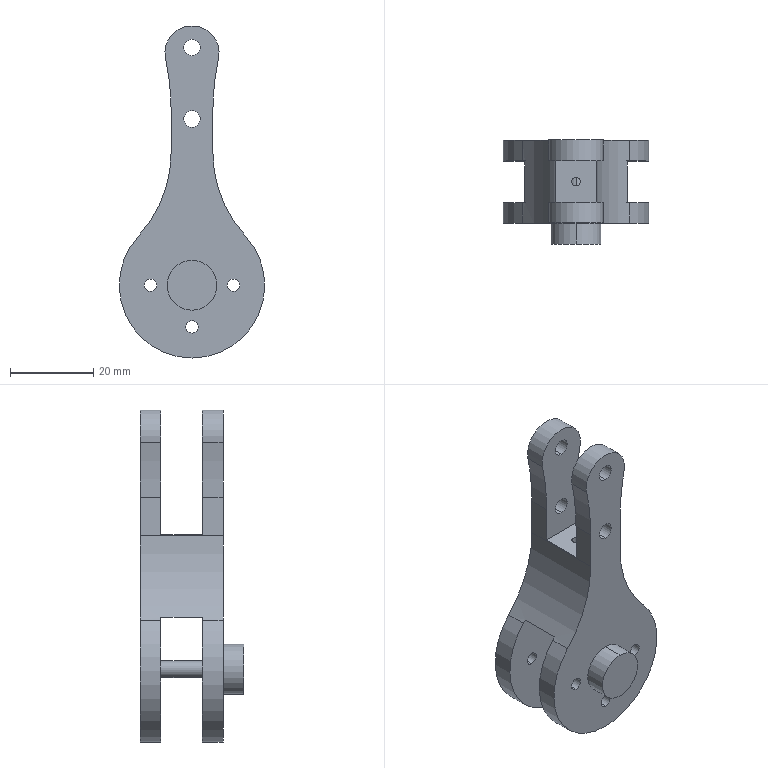Part | SolidWorks | features ICE 7, Extrusion 1 | 2 solids | 56 faces | box 35 x 25 x 79.915 mm | volume 17778 mm3 | cylinder 42 | plane 14 | commonest cylinder face diameters 4 x14 3 x12 35 x4 130 x4 2 x2 12 x2